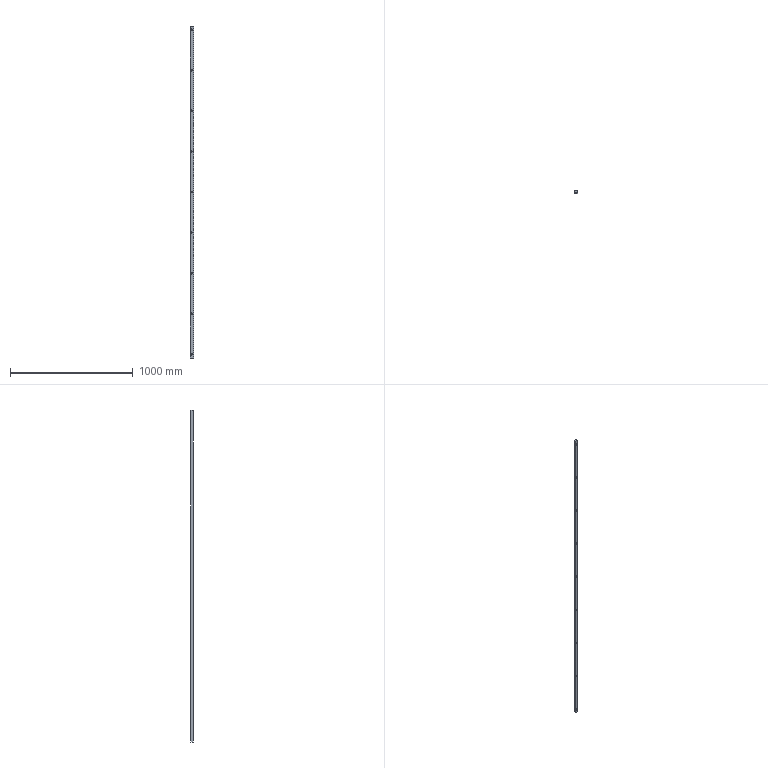Part | STEP file | PE_03 | 1 solid | 24 faces | box 25 x 20 x 2700 mm | volume 1341954 mm3 | cone 9 | cylinder 9 | plane 6 | commonest cylinder face diameters 6.5 x9